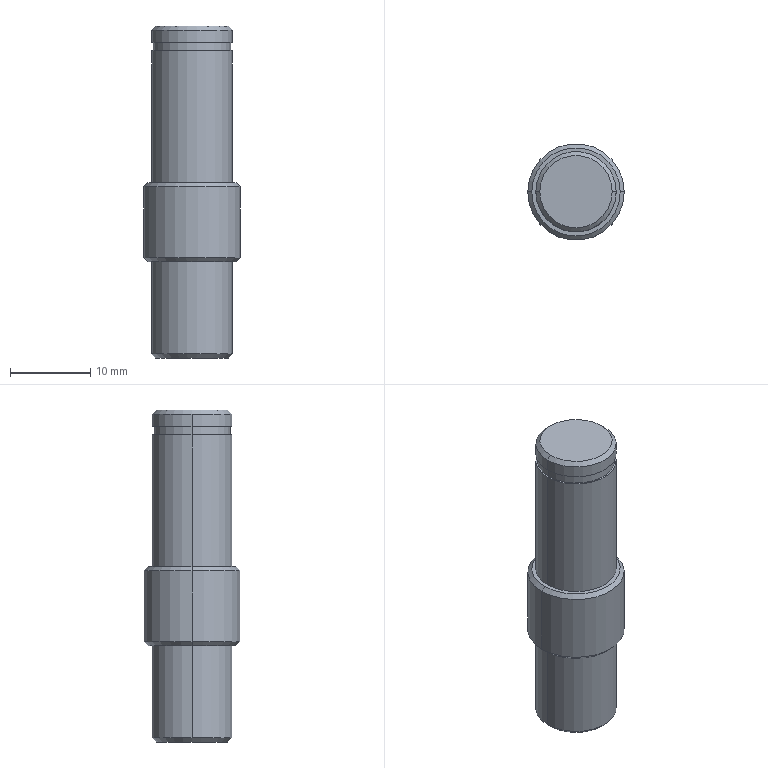Part | STEP file | PN_0034 Mount electronic clip support wheel shaft | 1 solid | 28 faces | box 12 x 12 x 41.3 mm | volume 3359 mm3 | cylinder 12 | cone 10 | plane 6 | commonest cylinder face diameters 10 x6 4.2 x2 9.6 x2 12 x2